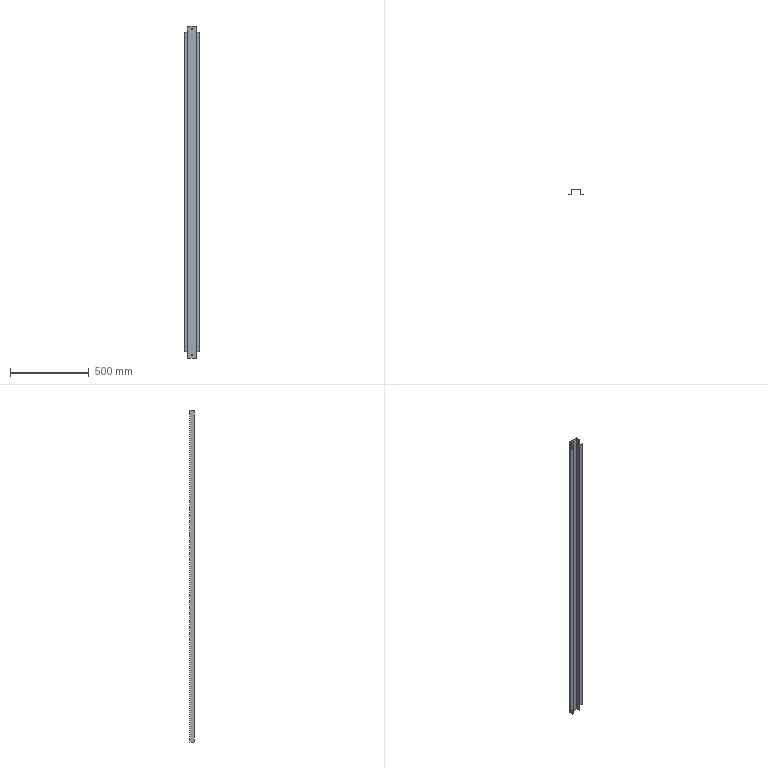Part | SolidWorks | features ICE 2, Chamfer 1, FlatPattern 1, MoveCopyBody 1, SMBaseFlange 1, SheetMetal 1 | 1 solid | 54 faces | box 100 x 30.8 x 2109 mm | volume 262992 mm3 | plane 42 | cylinder 12 | commonest cylinder face diameters 2 x4 3.6 x4 10 x4
STEP:
#1=CARTESIAN_POINT('',(0.,30.,1029.5));
#2=VERTEX_POINT('',#1);
#3=CARTESIAN_POINT('',(0.,30.,1039.5));
#4=VERTEX_POINT('',#3);
#5=CARTESIAN_POINT('',(0.,30.,1034.5));
#6=DIRECTION('',(0.,1.,0.));
#7=DIRECTION('',(-1.,0.,0.));
#8=AXIS2_PLACEMENT_3D('',#5,#6,#7);
#9=CIRCLE('',#8,5.);
#10=EDGE_CURVE('',#2,#4,#9,.T.);
#11=ORIENTED_EDGE('',*,*,#10,.F.);
#12=CARTESIAN_POINT('',(0.,30.8,1029.5));
#13=VERTEX_POINT('',#12);
#14=CARTESIAN_POINT('',(0.,20.8,1029.5));
#15=DIRECTION('',(0.,1.,0.));
#16=VECTOR('',#15,1000.);
#17=LINE('',#14,#16);
#18=EDGE_CURVE('',#2,#13,#17,.T.);
#19=ORIENTED_EDGE('',*,*,#18,.T.);
#20=CARTESIAN_POINT('',(0.,30.8,1039.5));
#21=VERTEX_POINT('',#20);
#22=CARTESIAN_POINT('',(0.,30.8,1034.5));
#23=DIRECTION('',(0.,1.,0.));
#24=DIRECTION('',(0.,0.,1.));
#25=AXIS2_PLACEMENT_3D('',#22,#23,#24);
#26=CIRCLE('',#25,5.);
#27=EDGE_CURVE('',#13,#21,#26,.T.);
#28=ORIENTED_EDGE('',*,*,#27,.T.);
#29=CARTESIAN_POINT('',(0.,20.8,1039.5));
#30=DIRECTION('',(0.,1.,0.));
#31=VECTOR('',#30,1000.);
#32=LINE('',#29,#31);
#33=EDGE_CURVE('',#4,#21,#32,.T.);
#34=ORIENTED_EDGE('',*,*,#33,.F.);
#35=EDGE_LOOP('',(#11,#19,#28,#34));
#36=FACE_OUTER_BOUND('',#35,.T.);
#37=CARTESIAN_POINT('',(0.,20.8,1034.5));
#38=DIRECTION('',(0.,1.,0.));
#39=DIRECTION('',(0.,0.,1.));
#40=AXIS2_PLACEMENT_3D('',#37,#38,#39);
#41=CYLINDRICAL_SURFACE('',#40,5.);
#42=ADVANCED_FACE('',(#36),#41,.F.);
#43=CARTESIAN_POINT('',(0.,30.,-1039.5));
#44=VERTEX_POINT('',#43);
#45=CARTESIAN_POINT('',(0.,30.,-1029.5));
#46=VERTEX_POINT('',#45);
#47=CARTESIAN_POINT('',(0.,30.,-1034.5));
#48=DIRECTION('',(0.,1.,0.));
#49=DIRECTION('',(-1.,0.,0.));
#50=AXIS2_PLACEMENT_3D('',#47,#48,#49);
#51=CIRCLE('',#50,5.);
#52=EDGE_CURVE('',#44,#46,#51,.T.);
#53=ORIENTED_EDGE('',*,*,#52,.F.);
#54=CARTESIAN_POINT('',(0.,30.8,-1039.5));
#55=VERTEX_POINT('',#54);
#56=CARTESIAN_POINT('',(0.,20.8,-1039.5));
#57=DIRECTION('',(0.,1.,0.));
#58=VECTOR('',#57,1000.);
#59=LINE('',#56,#58);
#60=EDGE_CURVE('',#44,#55,#59,.T.);
#61=ORIENTED_EDGE('',*,*,#60,.T.);
#62=CARTESIAN_POINT('',(0.,30.8,-1029.5));
#63=VERTEX_POINT('',#62);
#64=CARTESIAN_POINT('',(0.,30.8,-1034.5));
#65=DIRECTION('',(0.,1.,0.));
#66=DIRECTION('',(0.,0.,-1.));
#67=AXIS2_PLACEMENT_3D('',#64,#65,#66);
#68=CIRCLE('',#67,5.);
#69=EDGE_CURVE('',#55,#63,#68,.T.);
#70=ORIENTED_EDGE('',*,*,#69,.T.);
#71=CARTESIAN_POINT('',(0.,20.8,-1029.5));
#72=DIRECTION('',(0.,1.,0.));
#73=VECTOR('',#72,1000.);
#74=LINE('',#71,#73);
#75=EDGE_CURVE('',#46,#63,#74,.T.);
#76=ORIENTED_EDGE('',*,*,#75,.F.);
#77=EDGE_LOOP('',(#53,#61,#70,#76));
#78=FACE_OUTER_BOUND('',#77,.T.);
#79=CARTESIAN_POINT('',(0.,20.8,-1034.5));
#80=DIRECTION('',(0.,1.,0.));
#81=DIRECTION('',(0.,0.,1.));
#82=AXIS2_PLACEMENT_3D('',#79,#80,#81);
#83=CYLINDRICAL_SURFACE('',#82,5.);
#84=ADVANCED_FACE('',(#78),#83,.F.);
#85=CARTESIAN_POINT('',(-50.,0.,1014.5));
#86=VERTEX_POINT('',#85);
#87=CARTESIAN_POINT('',(-31.,0.,1014.5));
#88=VERTEX_POINT('',#87);
#89=CARTESIAN_POINT('',(-50.,0.,1014.5));
#90=DIRECTION('',(1.,0.,0.));
#91=VECTOR('',#90,1000.);
#92=LINE('',#89,#91);
#93=EDGE_CURVE('',#86,#88,#92,.T.);
#94=ORIENTED_EDGE('',*,*,#93,.T.);
#95=CARTESIAN_POINT('',(-31.,0.8,1014.5));
#96=VERTEX_POINT('',#95);
#97=CARTESIAN_POINT('',(-31.,0.,1014.5));
#98=DIRECTION('',(0.,1.,0.));
#99=VECTOR('',#98,1000.);
#100=LINE('',#97,#99);
#101=EDGE_CURVE('',#88,#96,#100,.T.);
#102=ORIENTED_EDGE('',*,*,#101,.T.);
#103=CARTESIAN_POINT('',(-50.,0.8,1014.5));
#104=VERTEX_POINT('',#103);
#105=CARTESIAN_POINT('',(-50.,0.8,1014.5));
#106=DIRECTION('',(-1.,0.,0.));
#107=VECTOR('',#106,1000.);
#108=LINE('',#105,#107);
#109=EDGE_CURVE('',#96,#104,#108,.T.);
#110=ORIENTED_EDGE('',*,*,#109,.T.);
#111=CARTESIAN_POINT('',(-50.,0.,1014.5));
#112=DIRECTION('',(0.,1.,0.));
#113=VECTOR('',#112,1000.);
#114=LINE('',#111,#113);
#115=EDGE_CURVE('',#86,#104,#114,.T.);
#116=ORIENTED_EDGE('',*,*,#115,.F.);
#117=EDGE_LOOP('',(#94,#102,#110,#116));
#118=FACE_OUTER_BOUND('',#117,.T.);
#119=CARTESIAN_POINT('',(-50.,0.,1014.5));
#120=DIRECTION('',(0.,0.,-1.));
#121=DIRECTION('',(-1.,0.,0.));
#122=AXIS2_PLACEMENT_3D('',#119,#120,#121);
#123=PLANE('',#122);
#124=ADVANCED_FACE('',(#118),#123,.F.);
#125=CARTESIAN_POINT('',(-30.,2.,1014.5));
#126=VERTEX_POINT('',#125);
#127=CARTESIAN_POINT('',(-30.,1.8,1014.5));
#128=VERTEX_POINT('',#127);
#129=CARTESIAN_POINT('',(-30.,0.8,1014.5));
#130=DIRECTION('',(0.,-1.,0.));
#131=VECTOR('',#130,1000.);
#132=LINE('',#129,#131);
#133=EDGE_CURVE('',#126,#128,#132,.T.);
#134=ORIENTED_EDGE('',*,*,#133,.T.);
#135=CARTESIAN_POINT('',(-29.2,1.8,1014.5));
#136=VERTEX_POINT('',#135);
#137=CARTESIAN_POINT('',(-30.,1.8,1014.5));
#138=DIRECTION('',(1.,0.,0.));
#139=VECTOR('',#138,1000.);
#140=LINE('',#137,#139);
#141=EDGE_CURVE('',#128,#136,#140,.T.);
#142=ORIENTED_EDGE('',*,*,#141,.T.);
#143=CARTESIAN_POINT('',(-29.2,2.,1014.5));
#144=VERTEX_POINT('',#143);
#145=CARTESIAN_POINT('',(-29.2,0.8,1014.5));
#146=DIRECTION('',(0.,-1.,0.));
#147=VECTOR('',#146,1000.);
#148=LINE('',#145,#147);
#149=EDGE_CURVE('',#144,#136,#148,.T.);
#150=ORIENTED_EDGE('',*,*,#149,.F.);
#151=CARTESIAN_POINT('',(-50.,2.,1014.5));
#152=DIRECTION('',(1.,0.,0.));
#153=VECTOR('',#152,1000.);
#154=LINE('',#151,#153);
#155=EDGE_CURVE('',#126,#144,#154,.T.);
#156=ORIENTED_EDGE('',*,*,#155,.F.);
#157=EDGE_LOOP('',(#134,#142,#150,#156));
#158=FACE_OUTER_BOUND('',#157,.T.);
#159=CARTESIAN_POINT('',(-50.,0.,1014.5));
#160=DIRECTION('',(0.,0.,-1.));
#161=DIRECTION('',(-1.,0.,0.));
#162=AXIS2_PLACEMENT_3D('',#159,#160,#161);
#163=PLANE('',#162);
#164=ADVANCED_FACE('',(#158),#163,.F.);
#165=CARTESIAN_POINT('',(-50.,0.8,-1014.5));
#166=VERTEX_POINT('',#165);
#167=CARTESIAN_POINT('',(-31.,0.8,-1014.5));
#168=VERTEX_POINT('',#167);
#169=CARTESIAN_POINT('',(-50.,0.8,-1014.5));
#170=DIRECTION('',(1.,0.,0.));
#171=VECTOR('',#170,1000.);
#172=LINE('',#169,#171);
#173=EDGE_CURVE('',#166,#168,#172,.T.);
#174=ORIENTED_EDGE('',*,*,#173,.T.);
#175=CARTESIAN_POINT('',(-31.,0.,-1014.5));
#176=VERTEX_POINT('',#175);
#177=CARTESIAN_POINT('',(-31.,0.8,-1014.5));
#178=DIRECTION('',(0.,-1.,0.));
#179=VECTOR('',#178,1000.);
#180=LINE('',#177,#179);
#181=EDGE_CURVE('',#168,#176,#180,.T.);
#182=ORIENTED_EDGE('',*,*,#181,.T.);
#183=CARTESIAN_POINT('',(-50.,0.,-1014.5));
#184=VERTEX_POINT('',#183);
#185=CARTESIAN_POINT('',(-50.,0.,-1014.5));
#186=DIRECTION('',(1.,0.,0.));
#187=VECTOR('',#186,1000.);
#188=LINE('',#185,#187);
#189=EDGE_CURVE('',#184,#176,#188,.T.);
#190=ORIENTED_EDGE('',*,*,#189,.F.);
#191=CARTESIAN_POINT('',(-50.,0.,-1014.5));
#192=DIRECTION('',(0.,-1.,0.));
#193=VECTOR('',#192,1000.);
#194=LINE('',#191,#193);
#195=EDGE_CURVE('',#166,#184,#194,.T.);
#196=ORIENTED_EDGE('',*,*,#195,.F.);
#197=EDGE_LOOP('',(#174,#182,#190,#196));
#198=FACE_OUTER_BOUND('',#197,.T.);
#199=CARTESIAN_POINT('',(-50.,0.,-1014.5));
#200=DIRECTION('',(0.,0.,1.));
#201=DIRECTION('',(1.,0.,0.));
#202=AXIS2_PLACEMENT_3D('',#199,#200,#201);
#203=PLANE('',#202);
#204=ADVANCED_FACE('',(#198),#203,.F.);
#205=CARTESIAN_POINT('',(-29.2,1.8,-1014.5));
#206=VERTEX_POINT('',#205);
#207=CARTESIAN_POINT('',(-29.2,2.,-1014.5));
#208=VERTEX_POINT('',#207);
#209=CARTESIAN_POINT('',(-29.2,0.8,-1014.5));
#210=DIRECTION('',(0.,1.,0.));
#211=VECTOR('',#210,1000.);
#212=LINE('',#209,#211);
#213=EDGE_CURVE('',#206,#208,#212,.T.);
#214=ORIENTED_EDGE('',*,*,#213,.F.);
#215=CARTESIAN_POINT('',(-30.,1.8,-1014.5));
#216=VERTEX_POINT('',#215);
#217=CARTESIAN_POINT('',(-29.2,1.8,-1014.5));
#218=DIRECTION('',(-1.,0.,0.));
#219=VECTOR('',#218,1000.);
#220=LINE('',#217,#219);
#221=EDGE_CURVE('',#206,#216,#220,.T.);
#222=ORIENTED_EDGE('',*,*,#221,.T.);
#223=CARTESIAN_POINT('',(-30.,2.,-1014.5));
#224=VERTEX_POINT('',#223);
#225=CARTESIAN_POINT('',(-30.,0.8,-1014.5));
#226=DIRECTION('',(0.,1.,0.));
#227=VECTOR('',#226,1000.);
#228=LINE('',#225,#227);
#229=EDGE_CURVE('',#216,#224,#228,.T.);
#230=ORIENTED_EDGE('',*,*,#229,.T.);
#231=CARTESIAN_POINT('',(-50.,2.,-1014.5));
#232=DIRECTION('',(1.,0.,0.));
#233=VECTOR('',#232,1000.);
#234=LINE('',#231,#233);
#235=EDGE_CURVE('',#224,#208,#234,.T.);
#236=ORIENTED_EDGE('',*,*,#235,.T.);
#237=EDGE_LOOP('',(#214,#222,#230,#236));
#238=FACE_OUTER_BOUND('',#237,.T.);
#239=CARTESIAN_POINT('',(-50.,0.,-1014.5));
#240=DIRECTION('',(0.,0.,1.));
#241=DIRECTION('',(1.,0.,0.));
#242=AXIS2_PLACEMENT_3D('',#239,#240,#241);
#243=PLANE('',#242);
#244=ADVANCED_FACE('',(#238),#243,.F.);
#245=CARTESIAN_POINT('',(29.2,1.8,1014.5));
#246=VERTEX_POINT('',#245);
#247=CARTESIAN_POINT('',(29.2,2.,1014.5));
#248=VERTEX_POINT('',#247);
#249=CARTESIAN_POINT('',(29.2,30.8,1014.5));
#250=DIRECTION('',(0.,1.,0.));
#251=VECTOR('',#250,1000.);
#252=LINE('',#249,#251);
#253=EDGE_CURVE('',#246,#248,#252,.T.);
#254=ORIENTED_EDGE('',*,*,#253,.F.);
#255=CARTESIAN_POINT('',(30.,1.8,1014.5));
#256=VERTEX_POINT('',#255);
#257=CARTESIAN_POINT('',(29.2,1.8,1014.5));
#258=DIRECTION('',(1.,0.,0.));
#259=VECTOR('',#258,1000.);
#260=LINE('',#257,#259);
#261=EDGE_CURVE('',#246,#256,#260,.T.);
#262=ORIENTED_EDGE('',*,*,#261,.T.);
#263=CARTESIAN_POINT('',(30.,2.,1014.5));
#264=VERTEX_POINT('',#263);
#265=CARTESIAN_POINT('',(30.,30.8,1014.5));
#266=DIRECTION('',(0.,1.,0.));
#267=VECTOR('',#266,1000.);
#268=LINE('',#265,#267);
#269=EDGE_CURVE('',#256,#264,#268,.T.);
#270=ORIENTED_EDGE('',*,*,#269,.T.);
#271=CARTESIAN_POINT('',(-50.,2.,1014.5));
#272=DIRECTION('',(1.,0.,0.));
#273=VECTOR('',#272,1000.);
#274=LINE('',#271,#273);
#275=EDGE_CURVE('',#248,#264,#274,.T.);
#276=ORIENTED_EDGE('',*,*,#275,.F.);
#277=EDGE_LOOP('',(#254,#262,#270,#276));
#278=FACE_OUTER_BOUND('',#277,.T.);
#279=CARTESIAN_POINT('',(-50.,0.,1014.5));
#280=DIRECTION('',(0.,0.,-1.));
#281=DIRECTION('',(-1.,0.,0.));
#282=AXIS2_PLACEMENT_3D('',#279,#280,#281);
#283=PLANE('',#282);
#284=ADVANCED_FACE('',(#278),#283,.F.);
#285=CARTESIAN_POINT('',(50.,0.8,1014.5));
#286=VERTEX_POINT('',#285);
#287=CARTESIAN_POINT('',(31.,0.8,1014.5));
#288=VERTEX_POINT('',#287);
#289=CARTESIAN_POINT('',(30.,0.8,1014.5));
#290=DIRECTION('',(-1.,0.,0.));
#291=VECTOR('',#290,1000.);
#292=LINE('',#289,#291);
#293=EDGE_CURVE('',#286,#288,#292,.T.);
#294=ORIENTED_EDGE('',*,*,#293,.T.);
#295=CARTESIAN_POINT('',(31.,0.,1014.5));
#296=VERTEX_POINT('',#295);
#297=CARTESIAN_POINT('',(31.,0.8,1014.5));
#298=DIRECTION('',(0.,-1.,0.));
#299=VECTOR('',#298,1000.);
#300=LINE('',#297,#299);
#301=EDGE_CURVE('',#288,#296,#300,.T.);
#302=ORIENTED_EDGE('',*,*,#301,.T.);
#303=CARTESIAN_POINT('',(50.,0.,1014.5));
#304=VERTEX_POINT('',#303);
#305=CARTESIAN_POINT('',(-50.,0.,1014.5));
#306=DIRECTION('',(1.,0.,0.));
#307=VECTOR('',#306,1000.);
#308=LINE('',#305,#307);
#309=EDGE_CURVE('',#296,#304,#308,.T.);
#310=ORIENTED_EDGE('',*,*,#309,.T.);
#311=CARTESIAN_POINT('',(50.,0.,1014.5));
#312=DIRECTION('',(0.,1.,0.));
#313=VECTOR('',#312,1000.);
#314=LINE('',#311,#313);
#315=EDGE_CURVE('',#304,#286,#314,.T.);
#316=ORIENTED_EDGE('',*,*,#315,.T.);
#317=EDGE_LOOP('',(#294,#302,#310,#316));
#318=FACE_OUTER_BOUND('',#317,.T.);
#319=CARTESIAN_POINT('',(-50.,0.,1014.5));
#320=DIRECTION('',(0.,0.,-1.));
#321=DIRECTION('',(-1.,0.,0.));
#322=AXIS2_PLACEMENT_3D('',#319,#320,#321);
#323=PLANE('',#322);
#324=ADVANCED_FACE('',(#318),#323,.F.);
#325=CARTESIAN_POINT('',(30.,2.,-1014.5));
#326=VERTEX_POINT('',#325);
#327=CARTESIAN_POINT('',(30.,1.8,-1014.5));
#328=VERTEX_POINT('',#327);
#329=CARTESIAN_POINT('',(30.,30.8,-1014.5));
#330=DIRECTION('',(0.,-1.,0.));
#331=VECTOR('',#330,1000.);
#332=LINE('',#329,#331);
#333=EDGE_CURVE('',#326,#328,#332,.T.);
#334=ORIENTED_EDGE('',*,*,#333,.T.);
#335=CARTESIAN_POINT('',(29.2,1.8,-1014.5));
#336=VERTEX_POINT('',#335);
#337=CARTESIAN_POINT('',(30.,1.8,-1014.5));
#338=DIRECTION('',(-1.,0.,0.));
#339=VECTOR('',#338,1000.);
#340=LINE('',#337,#339);
#341=EDGE_CURVE('',#328,#336,#340,.T.);
#342=ORIENTED_EDGE('',*,*,#341,.T.);
#343=CARTESIAN_POINT('',(29.2,2.,-1014.5));
#344=VERTEX_POINT('',#343);
#345=CARTESIAN_POINT('',(29.2,30.8,-1014.5));
#346=DIRECTION('',(0.,-1.,0.));
#347=VECTOR('',#346,1000.);
#348=LINE('',#345,#347);
#349=EDGE_CURVE('',#344,#336,#348,.T.);
#350=ORIENTED_EDGE('',*,*,#349,.F.);
#351=CARTESIAN_POINT('',(-50.,2.,-1014.5));
#352=DIRECTION('',(1.,0.,0.));
#353=VECTOR('',#352,1000.);
#354=LINE('',#351,#353);
#355=EDGE_CURVE('',#344,#326,#354,.T.);
#356=ORIENTED_EDGE('',*,*,#355,.T.);
#357=EDGE_LOOP('',(#334,#342,#350,#356));
#358=FACE_OUTER_BOUND('',#357,.T.);
#359=CARTESIAN_POINT('',(-50.,0.,-1014.5));
#360=DIRECTION('',(0.,0.,1.));
#361=DIRECTION('',(1.,0.,0.));
#362=AXIS2_PLACEMENT_3D('',#359,#360,#361);
#363=PLANE('',#362);
#364=ADVANCED_FACE('',(#358),#363,.F.);
#365=CARTESIAN_POINT('',(31.,0.,-1014.5));
#366=VERTEX_POINT('',#365);
#367=CARTESIAN_POINT('',(50.,0.,-1014.5));
#368=VERTEX_POINT('',#367);
#369=CARTESIAN_POINT('',(-50.,0.,-1014.5));
#370=DIRECTION('',(1.,0.,0.));
#371=VECTOR('',#370,1000.);
#372=LINE('',#369,#371);
#373=EDGE_CURVE('',#366,#368,#372,.T.);
#374=ORIENTED_EDGE('',*,*,#373,.F.);
#375=CARTESIAN_POINT('',(31.,0.8,-1014.5));
#376=VERTEX_POINT('',#375);
#377=CARTESIAN_POINT('',(31.,0.,-1014.5));
#378=DIRECTION('',(0.,1.,0.));
#379=VECTOR('',#378,1000.);
#380=LINE('',#377,#379);
#381=EDGE_CURVE('',#366,#376,#380,.T.);
#382=ORIENTED_EDGE('',*,*,#381,.T.);
#383=CARTESIAN_POINT('',(50.,0.8,-1014.5));
#384=VERTEX_POINT('',#383);
#385=CARTESIAN_POINT('',(30.,0.8,-1014.5));
#386=DIRECTION('',(1.,0.,0.));
#387=VECTOR('',#386,1000.);
#388=LINE('',#385,#387);
#389=EDGE_CURVE('',#376,#384,#388,.T.);
#390=ORIENTED_EDGE('',*,*,#389,.T.);
#391=CARTESIAN_POINT('',(50.,0.,-1014.5));
#392=DIRECTION('',(0.,-1.,0.));
#393=VECTOR('',#392,1000.);
#394=LINE('',#391,#393);
#395=EDGE_CURVE('',#384,#368,#394,.T.);
#396=ORIENTED_EDGE('',*,*,#395,.T.);
#397=EDGE_LOOP('',(#374,#382,#390,#396));
#398=FACE_OUTER_BOUND('',#397,.T.);
#399=CARTESIAN_POINT('',(-50.,0.,-1014.5));
#400=DIRECTION('',(0.,0.,1.));
#401=DIRECTION('',(1.,0.,0.));
#402=AXIS2_PLACEMENT_3D('',#399,#400,#401);
#403=PLANE('',#402);
#404=ADVANCED_FACE('',(#398),#403,.F.);
#405=CARTESIAN_POINT('',(-30.,7.,1054.5));
#406=VERTEX_POINT('',#405);
#407=CARTESIAN_POINT('',(-30.,29.,1054.5));
#408=VERTEX_POINT('',#407);
#409=CARTESIAN_POINT('',(-30.,0.8,1054.5));
#410=DIRECTION('',(0.,1.,0.));
#411=VECTOR('',#410,1000.);
#412=LINE('',#409,#411);
#413=EDGE_CURVE('',#406,#408,#412,.T.);
#414=ORIENTED_EDGE('',*,*,#413,.F.);
#415=CARTESIAN_POINT('',(-29.2,7.,1054.5));
#416=VERTEX_POINT('',#415);
#417=CARTESIAN_POINT('',(-29.2,7.,1054.5));
#418=DIRECTION('',(1.,0.,0.));
#419=VECTOR('',#418,1000.);
#420=LINE('',#417,#419);
#421=EDGE_CURVE('',#406,#416,#420,.T.);
#422=ORIENTED_EDGE('',*,*,#421,.T.);
#423=CARTESIAN_POINT('',(-29.2,29.,1054.5));
#424=VERTEX_POINT('',#423);
#425=CARTESIAN_POINT('',(-29.2,0.8,1054.5));
#426=DIRECTION('',(0.,1.,0.));
#427=VECTOR('',#426,1000.);
#428=LINE('',#425,#427);
#429=EDGE_CURVE('',#416,#424,#428,.T.);
#430=ORIENTED_EDGE('',*,*,#429,.T.);
#431=CARTESIAN_POINT('',(-29.2,29.,1054.5));
#432=DIRECTION('',(-1.,0.,0.));
#433=VECTOR('',#432,1000.);
#434=LINE('',#431,#433);
#435=EDGE_CURVE('',#424,#408,#434,.T.);
#436=ORIENTED_EDGE('',*,*,#435,.T.);
#437=EDGE_LOOP('',(#414,#422,#430,#436));
#438=FACE_OUTER_BOUND('',#437,.T.);
#439=CARTESIAN_POINT('',(-31.,0.,1054.5));
#440=DIRECTION('',(0.,0.,1.));
#441=DIRECTION('',(1.,0.,0.));
#442=AXIS2_PLACEMENT_3D('',#439,#440,#441);
#443=PLANE('',#442);
#444=ADVANCED_FACE('',(#438),#443,.T.);
#445=CARTESIAN_POINT('',(-28.2,30.8,1054.5));
#446=VERTEX_POINT('',#445);
#447=CARTESIAN_POINT('',(-28.2,30.,1054.5));
#448=VERTEX_POINT('',#447);
#449=CARTESIAN_POINT('',(-28.2,30.8,1054.5));
#450=DIRECTION('',(0.,-1.,0.));
#451=VECTOR('',#450,1000.);
#452=LINE('',#449,#451);
#453=EDGE_CURVE('',#446,#448,#452,.T.);
#454=ORIENTED_EDGE('',*,*,#453,.F.);
#455=CARTESIAN_POINT('',(-28.2,29.,1054.5));
#456=DIRECTION('',(0.,0.,-1.));
#457=DIRECTION('',(1.,0.,0.));
#458=AXIS2_PLACEMENT_3D('',#455,#456,#457);
#459=CIRCLE('',#458,1.8);
#460=EDGE_CURVE('',#408,#446,#459,.T.);
#461=ORIENTED_EDGE('',*,*,#460,.F.);
#462=ORIENTED_EDGE('',*,*,#435,.F.);
#463=CARTESIAN_POINT('',(-28.2,29.,1054.5));
#464=DIRECTION('',(0.,0.,-1.));
#465=DIRECTION('',(1.,0.,0.));
#466=AXIS2_PLACEMENT_3D('',#463,#464,#465);
#467=CIRCLE('',#466,1.);
#468=EDGE_CURVE('',#424,#448,#467,.T.);
#469=ORIENTED_EDGE('',*,*,#468,.T.);
#470=EDGE_LOOP('',(#454,#461,#462,#469));
#471=FACE_OUTER_BOUND('',#470,.T.);
#472=CARTESIAN_POINT('',(-28.2,30.8,1054.5));
#473=DIRECTION('',(0.,0.,1.));
#474=DIRECTION('',(1.,0.,0.));
#475=AXIS2_PLACEMENT_3D('',#472,#473,#474);
#476=PLANE('',#475);
#477=ADVANCED_FACE('',(#471),#476,.T.);
#478=CARTESIAN_POINT('',(28.2,30.8,1054.5));
#479=VERTEX_POINT('',#478);
#480=CARTESIAN_POINT('',(-30.,30.8,1054.5));
#481=DIRECTION('',(1.,0.,0.));
#482=VECTOR('',#481,1000.);
#483=LINE('',#480,#482);
#484=EDGE_CURVE('',#446,#479,#483,.T.);
#485=ORIENTED_EDGE('',*,*,#484,.F.);
#486=ORIENTED_EDGE('',*,*,#453,.T.);
#487=CARTESIAN_POINT('',(28.2,30.,1054.5));
#488=VERTEX_POINT('',#487);
#489=CARTESIAN_POINT('',(-30.,30.,1054.5));
#490=DIRECTION('',(1.,0.,0.));
#491=VECTOR('',#490,1000.);
#492=LINE('',#489,#491);
#493=EDGE_CURVE('',#448,#488,#492,.T.);
#494=ORIENTED_EDGE('',*,*,#493,.T.);
#495=CARTESIAN_POINT('',(28.2,30.,1054.5));
#496=DIRECTION('',(0.,1.,0.));
#497=VECTOR('',#496,1000.);
#498=LINE('',#495,#497);
#499=EDGE_CURVE('',#488,#479,#498,.T.);
#500=ORIENTED_EDGE('',*,*,#499,.T.);
#501=EDGE_LOOP('',(#485,#486,#494,#500));
#502=FACE_OUTER_BOUND('',#501,.T.);
#503=CARTESIAN_POINT('',(-29.2,29.,1054.5));
#504=DIRECTION('',(0.,0.,1.));
#505=DIRECTION('',(1.,0.,0.));
#506=AXIS2_PLACEMENT_3D('',#503,#504,#505);
#507=PLANE('',#506);
#508=ADVANCED_FACE('',(#502),#507,.T.);
#509=CARTESIAN_POINT('',(-30.,29.,-1054.5));
#510=VERTEX_POINT('',#509);
#511=CARTESIAN_POINT('',(-29.2,29.,-1054.5));
#512=VERTEX_POINT('',#511);
#513=CARTESIAN_POINT('',(-30.,29.,-1054.5));
#514=DIRECTION('',(1.,0.,0.));
#515=VECTOR('',#514,1000.);
#516=LINE('',#513,#515);
#517=EDGE_CURVE('',#510,#512,#516,.T.);
#518=ORIENTED_EDGE('',*,*,#517,.F.);
#519=CARTESIAN_POINT('',(-28.2,30.8,-1054.5));
#520=VERTEX_POINT('',#519);
#521=CARTESIAN_POINT('',(-28.2,29.,-1054.5));
#522=DIRECTION('',(0.,0.,-1.));
#523=DIRECTION('',(1.,0.,0.));
#524=AXIS2_PLACEMENT_3D('',#521,#522,#523);
#525=CIRCLE('',#524,1.8);
#526=EDGE_CURVE('',#510,#520,#525,.T.);
#527=ORIENTED_EDGE('',*,*,#526,.T.);
#528=CARTESIAN_POINT('',(-28.2,30.,-1054.5));
#529=VERTEX_POINT('',#528);
#530=CARTESIAN_POINT('',(-28.2,30.,-1054.5));
#531=DIRECTION('',(0.,1.,0.));
#532=VECTOR('',#531,1000.);
#533=LINE('',#530,#532);
#534=EDGE_CURVE('',#529,#520,#533,.T.);
#535=ORIENTED_EDGE('',*,*,#534,.F.);
#536=CARTESIAN_POINT('',(-28.2,29.,-1054.5));
#537=DIRECTION('',(0.,0.,-1.));
#538=DIRECTION('',(1.,0.,0.));
#539=AXIS2_PLACEMENT_3D('',#536,#537,#538);
#540=CIRCLE('',#539,1.);
#541=EDGE_CURVE('',#512,#529,#540,.T.);
#542=ORIENTED_EDGE('',*,*,#541,.F.);
#543=EDGE_LOOP('',(#518,#527,#535,#542));
#544=FACE_OUTER_BOUND('',#543,.T.);
#545=CARTESIAN_POINT('',(-30.,29.,-1054.5));
#546=DIRECTION('',(0.,0.,-1.));
#547=DIRECTION('',(-1.,0.,0.));
#548=AXIS2_PLACEMENT_3D('',#545,#546,#547);
#549=PLANE('',#548);
#550=ADVANCED_FACE('',(#544),#549,.T.);
#551=CARTESIAN_POINT('',(-29.2,7.,-1054.5));
#552=VERTEX_POINT('',#551);
#553=CARTESIAN_POINT('',(-29.2,0.8,-1054.5));
#554=DIRECTION('',(0.,1.,0.));
#555=VECTOR('',#554,1000.);
#556=LINE('',#553,#555);
#557=EDGE_CURVE('',#552,#512,#556,.T.);
#558=ORIENTED_EDGE('',*,*,#557,.F.);
#559=CARTESIAN_POINT('',(-30.,7.,-1054.5));
#560=VERTEX_POINT('',#559);
#561=CARTESIAN_POINT('',(-30.,7.,-1054.5));
#562=DIRECTION('',(-1.,0.,0.));
#563=VECTOR('',#562,1000.);
#564=LINE('',#561,#563);
#565=EDGE_CURVE('',#552,#560,#564,.T.);
#566=ORIENTED_EDGE('',*,*,#565,.T.);
#567=CARTESIAN_POINT('',(-30.,0.8,-1054.5));
#568=DIRECTION('',(0.,1.,0.));
#569=VECTOR('',#568,1000.);
#570=LINE('',#567,#569);
#571=EDGE_CURVE('',#560,#510,#570,.T.);
#572=ORIENTED_EDGE('',*,*,#571,.T.);
#573=ORIENTED_EDGE('',*,*,#517,.T.);
#574=EDGE_LOOP('',(#558,#566,#572,#573));
#575=FACE_OUTER_BOUND('',#574,.T.);
#576=CARTESIAN_POINT('',(-28.2,30.,-1054.5));
#577=DIRECTION('',(0.,0.,-1.));
#578=DIRECTION('',(-1.,0.,0.));
#579=AXIS2_PLACEMENT_3D('',#576,#577,#578);
#580=PLANE('',#579);
#581=ADVANCED_FACE('',(#575),#580,.T.);
#582=CARTESIAN_POINT('',(30.,29.,1054.5));
#583=VERTEX_POINT('',#582);
#584=CARTESIAN_POINT('',(29.2,29.,1054.5));
#585=VERTEX_POINT('',#584);
#586=CARTESIAN_POINT('',(30.,29.,1054.5));
#587=DIRECTION('',(-1.,0.,0.));
#588=VECTOR('',#587,1000.);
#589=LINE('',#586,#588);
#590=EDGE_CURVE('',#583,#585,#589,.T.);
#591=ORIENTED_EDGE('',*,*,#590,.F.);
#592=CARTESIAN_POINT('',(28.2,29.,1054.5));
#593=DIRECTION('',(0.,0.,-1.));
#594=DIRECTION('',(1.,0.,0.));
#595=AXIS2_PLACEMENT_3D('',#592,#593,#594);
#596=CIRCLE('',#595,1.8);
#597=EDGE_CURVE('',#479,#583,#596,.T.);
#598=ORIENTED_EDGE('',*,*,#597,.F.);
#599=ORIENTED_EDGE('',*,*,#499,.F.);
#600=CARTESIAN_POINT('',(28.2,29.,1054.5));
#601=DIRECTION('',(0.,0.,-1.));
#602=DIRECTION('',(1.,0.,0.));
#603=AXIS2_PLACEMENT_3D('',#600,#601,#602);
#604=CIRCLE('',#603,1.);
#605=EDGE_CURVE('',#488,#585,#604,.T.);
#606=ORIENTED_EDGE('',*,*,#605,.T.);
#607=EDGE_LOOP('',(#591,#598,#599,#606));
#608=FACE_OUTER_BOUND('',#607,.T.);
#609=CARTESIAN_POINT('',(30.,29.,1054.5));
#610=DIRECTION('',(0.,0.,1.));
#611=DIRECTION('',(1.,0.,0.));
#612=AXIS2_PLACEMENT_3D('',#609,#610,#611);
#613=PLANE('',#612);
#614=ADVANCED_FACE('',(#608),#613,.T.);
#615=CARTESIAN_POINT('',(29.2,7.,1054.5));
#616=VERTEX_POINT('',#615);
#617=CARTESIAN_POINT('',(29.2,30.8,1054.5));
#618=DIRECTION('',(0.,-1.,0.));
#619=VECTOR('',#618,1000.);
#620=LINE('',#617,#619);
#621=EDGE_CURVE('',#585,#616,#620,.T.);
#622=ORIENTED_EDGE('',*,*,#621,.T.);
#623=CARTESIAN_POINT('',(30.,7.,1054.5));
#624=VERTEX_POINT('',#623);
#625=CARTESIAN_POINT('',(30.,7.,1054.5));
#626=DIRECTION('',(1.,0.,0.));
#627=VECTOR('',#626,1000.);
#628=LINE('',#625,#627);
#629=EDGE_CURVE('',#616,#624,#628,.T.);
#630=ORIENTED_EDGE('',*,*,#629,.T.);
#631=CARTESIAN_POINT('',(30.,30.8,1054.5));
#632=DIRECTION('',(0.,-1.,0.));
#633=VECTOR('',#632,1000.);
#634=LINE('',#631,#633);
#635=EDGE_CURVE('',#583,#624,#634,.T.);
#636=ORIENTED_EDGE('',*,*,#635,.F.);
#637=ORIENTED_EDGE('',*,*,#590,.T.);
#638=EDGE_LOOP('',(#622,#630,#636,#637));
#639=FACE_OUTER_BOUND('',#638,.T.);
#640=CARTESIAN_POINT('',(28.2,30.,1054.5));
#641=DIRECTION('',(0.,0.,1.));
#642=DIRECTION('',(1.,0.,0.));
#643=AXIS2_PLACEMENT_3D('',#640,#641,#642);
#644=PLANE('',#643);
#645=ADVANCED_FACE('',(#639),#644,.T.);
#646=CARTESIAN_POINT('',(28.2,30.8,-1054.5));
#647=VERTEX_POINT('',#646);
#648=CARTESIAN_POINT('',(28.2,30.,-1054.5));
#649=VERTEX_POINT('',#648);
#650=CARTESIAN_POINT('',(28.2,30.8,-1054.5));
#651=DIRECTION('',(0.,-1.,0.));
#652=VECTOR('',#651,1000.);
#653=LINE('',#650,#652);
#654=EDGE_CURVE('',#647,#649,#653,.T.);
#655=ORIENTED_EDGE('',*,*,#654,.F.);
#656=CARTESIAN_POINT('',(30.,29.,-1054.5));
#657=VERTEX_POINT('',#656);
#658=CARTESIAN_POINT('',(28.2,29.,-1054.5));
#659=DIRECTION('',(0.,0.,-1.));
#660=DIRECTION('',(1.,0.,0.));
#661=AXIS2_PLACEMENT_3D('',#658,#659,#660);
#662=CIRCLE('',#661,1.8);
#663=EDGE_CURVE('',#647,#657,#662,.T.);
#664=ORIENTED_EDGE('',*,*,#663,.T.);
#665=CARTESIAN_POINT('',(29.2,29.,-1054.5));
#666=VERTEX_POINT('',#665);
#667=CARTESIAN_POINT('',(29.2,29.,-1054.5));
#668=DIRECTION('',(1.,0.,0.));
#669=VECTOR('',#668,1000.);
#670=LINE('',#667,#669);
#671=EDGE_CURVE('',#666,#657,#670,.T.);
#672=ORIENTED_EDGE('',*,*,#671,.F.);
#673=CARTESIAN_POINT('',(28.2,29.,-1054.5));
#674=DIRECTION('',(0.,0.,-1.));
#675=DIRECTION('',(1.,0.,0.));
#676=AXIS2_PLACEMENT_3D('',#673,#674,#675);
#677=CIRCLE('',#676,1.);
#678=EDGE_CURVE('',#649,#666,#677,.T.);
#679=ORIENTED_EDGE('',*,*,#678,.F.);
#680=EDGE_LOOP('',(#655,#664,#672,#679));
#681=FACE_OUTER_BOUND('',#680,.T.);
#682=CARTESIAN_POINT('',(28.2,30.8,-1054.5));
#683=DIRECTION('',(0.,0.,-1.));
#684=DIRECTION('',(-1.,0.,0.));
#685=AXIS2_PLACEMENT_3D('',#682,#683,#684);
#686=PLANE('',#685);
#687=ADVANCED_FACE('',(#681),#686,.T.);
#688=CARTESIAN_POINT('',(-30.,30.8,-1054.5));
#689=DIRECTION('',(1.,0.,0.));
#690=VECTOR('',#689,1000.);
#691=LINE('',#688,#690);
#692=EDGE_CURVE('',#520,#647,#691,.T.);
#693=ORIENTED_EDGE('',*,*,#692,.T.);
#694=ORIENTED_EDGE('',*,*,#654,.T.);
#695=CARTESIAN_POINT('',(-30.,30.,-1054.5));
#696=DIRECTION('',(1.,0.,0.));
#697=VECTOR('',#696,1000.);
#698=LINE('',#695,#697);
#699=EDGE_CURVE('',#529,#649,#698,.T.);
#700=ORIENTED_EDGE('',*,*,#699,.F.);
#701=ORIENTED_EDGE('',*,*,#534,.T.);
#702=EDGE_LOOP('',(#693,#694,#700,#701));
#703=FACE_OUTER_BOUND('',#702,.T.);
#704=CARTESIAN_POINT('',(29.2,29.,-1054.5));
#705=DIRECTION('',(0.,0.,-1.));
#706=DIRECTION('',(-1.,0.,0.));
#707=AXIS2_PLACEMENT_3D('',#704,#705,#706);
#708=PLANE('',#707);
#709=ADVANCED_FACE('',(#703),#708,.T.);
#710=CARTESIAN_POINT('',(30.,7.,-1054.5));
#711=VERTEX_POINT('',#710);
#712=CARTESIAN_POINT('',(30.,30.8,-1054.5));
#713=DIRECTION('',(0.,-1.,0.));
#714=VECTOR('',#713,1000.);
#715=LINE('',#712,#714);
#716=EDGE_CURVE('',#657,#711,#715,.T.);
#717=ORIENTED_EDGE('',*,*,#716,.T.);
#718=CARTESIAN_POINT('',(29.2,7.,-1054.5));
#719=VERTEX_POINT('',#718);
#720=CARTESIAN_POINT('',(29.2,7.,-1054.5));
#721=DIRECTION('',(-1.,0.,0.));
#722=VECTOR('',#721,1000.);
#723=LINE('',#720,#722);
#724=EDGE_CURVE('',#711,#719,#723,.T.);
#725=ORIENTED_EDGE('',*,*,#724,.T.);
#726=CARTESIAN_POINT('',(29.2,30.8,-1054.5));
#727=DIRECTION('',(0.,-1.,0.));
#728=VECTOR('',#727,1000.);
#729=LINE('',#726,#728);
#730=EDGE_CURVE('',#666,#719,#729,.T.);
#731=ORIENTED_EDGE('',*,*,#730,.F.);
#732=ORIENTED_EDGE('',*,*,#671,.T.);
#733=EDGE_LOOP('',(#717,#725,#731,#732));
#734=FACE_OUTER_BOUND('',#733,.T.);
#735=CARTESIAN_POINT('',(31.,0.,-1054.5));
#736=DIRECTION('',(0.,0.,-1.));
#737=DIRECTION('',(-1.,0.,0.));
#738=AXIS2_PLACEMENT_3D('',#735,#736,#737);
#739=PLANE('',#738);
#740=ADVANCED_FACE('',(#734),#739,.T.);
#741=CARTESIAN_POINT('',(50.,0.,1054.5));
#742=DIRECTION('',(0.,0.,-1.));
#743=VECTOR('',#742,1000.);
#744=LINE('',#741,#743);
#745=EDGE_CURVE('',#304,#368,#744,.T.);
#746=ORIENTED_EDGE('',*,*,#745,.F.);
#747=ORIENTED_EDGE('',*,*,#309,.F.);
#748=CARTESIAN_POINT('',(31.,0.,1054.5));
#749=DIRECTION('',(0.,0.,-1.));
#750=VECTOR('',#749,1000.);
#751=LINE('',#748,#750);
#752=EDGE_CURVE('',#296,#366,#751,.T.);
#753=ORIENTED_EDGE('',*,*,#752,.T.);
#754=ORIENTED_EDGE('',*,*,#373,.T.);
#755=EDGE_LOOP('',(#746,#747,#753,#754));
#756=FACE_OUTER_BOUND('',#755,.T.);
#757=CARTESIAN_POINT('',(30.,0.,1054.5));
#758=DIRECTION('',(0.,1.,0.));
#759=DIRECTION('',(-1.,0.,0.));
#760=AXIS2_PLACEMENT_3D('',#757,#758,#759);
#761=PLANE('',#760);
#762=ADVANCED_FACE('',(#756),#761,.F.);
#763=ORIENTED_EDGE('',*,*,#315,.F.);
#764=ORIENTED_EDGE('',*,*,#745,.T.);
#765=ORIENTED_EDGE('',*,*,#395,.F.);
#766=CARTESIAN_POINT('',(50.,0.8,1054.5));
#767=DIRECTION('',(0.,0.,-1.));
#768=VECTOR('',#767,1000.);
#769=LINE('',#766,#768);
#770=EDGE_CURVE('',#286,#384,#769,.T.);
#771=ORIENTED_EDGE('',*,*,#770,.F.);
#772=EDGE_LOOP('',(#763,#764,#765,#771));
#773=FACE_OUTER_BOUND('',#772,.T.);
#774=CARTESIAN_POINT('',(50.,0.8,1054.5));
#775=DIRECTION('',(1.,0.,0.));
#776=DIRECTION('',(0.,0.,-1.));
#777=AXIS2_PLACEMENT_3D('',#774,#775,#776);
#778=PLANE('',#777);
#779=ADVANCED_FACE('',(#773),#778,.T.);
#780=ORIENTED_EDGE('',*,*,#293,.F.);
#781=ORIENTED_EDGE('',*,*,#770,.T.);
#782=ORIENTED_EDGE('',*,*,#389,.F.);
#783=CARTESIAN_POINT('',(31.,0.8,1054.5));
#784=DIRECTION('',(0.,0.,-1.));
#785=VECTOR('',#784,1000.);
#786=LINE('',#783,#785);
#787=EDGE_CURVE('',#288,#376,#786,.T.);
#788=ORIENTED_EDGE('',*,*,#787,.F.);
#789=EDGE_LOOP('',(#780,#781,#782,#788));
#790=FACE_OUTER_BOUND('',#789,.T.);
#791=CARTESIAN_POINT('',(30.,0.8,1054.5));
#792=DIRECTION('',(0.,1.,0.));
#793=DIRECTION('',(-1.,0.,0.));
#794=AXIS2_PLACEMENT_3D('',#791,#792,#793);
#795=PLANE('',#794);
#796=ADVANCED_FACE('',(#790),#795,.T.);
#797=CARTESIAN_POINT('',(31.,1.8,1014.5));
#798=DIRECTION('',(0.,0.,-1.));
#799=DIRECTION('',(-1.,0.,0.));
#800=AXIS2_PLACEMENT_3D('',#797,#798,#799);
#801=CIRCLE('',#800,1.);
#802=EDGE_CURVE('',#288,#256,#801,.T.);
#803=ORIENTED_EDGE('',*,*,#802,.F.);
#804=ORIENTED_EDGE('',*,*,#787,.T.);
#805=CARTESIAN_POINT('',(31.,1.8,-1014.5));
#806=DIRECTION('',(0.,0.,1.));
#807=DIRECTION('',(1.,0.,0.));
#808=AXIS2_PLACEMENT_3D('',#805,#806,#807);
#809=CIRCLE('',#808,1.);
#810=EDGE_CURVE('',#328,#376,#809,.T.);
#811=ORIENTED_EDGE('',*,*,#810,.F.);
#812=CARTESIAN_POINT('',(30.,1.8,1054.5));
#813=DIRECTION('',(0.,0.,-1.));
#814=VECTOR('',#813,1000.);
#815=LINE('',#812,#814);
#816=EDGE_CURVE('',#256,#328,#815,.T.);
#817=ORIENTED_EDGE('',*,*,#816,.F.);
#818=EDGE_LOOP('',(#803,#804,#811,#817));
#819=FACE_OUTER_BOUND('',#818,.T.);
#820=CARTESIAN_POINT('',(31.,1.8,1054.5));
#821=DIRECTION('',(0.,0.,-1.));
#822=DIRECTION('',(-1.,0.,0.));
#823=AXIS2_PLACEMENT_3D('',#820,#821,#822);
#824=CYLINDRICAL_SURFACE('',#823,1.);
#825=ADVANCED_FACE('',(#819),#824,.F.);
#826=CARTESIAN_POINT('',(30.,2.,-1049.5));
#827=VERTEX_POINT('',#826);
#828=CARTESIAN_POINT('',(30.,2.,1054.5));
#829=DIRECTION('',(0.,0.,1.));
#830=VECTOR('',#829,1000.);
#831=LINE('',#828,#830);
#832=EDGE_CURVE('',#827,#326,#831,.T.);
#833=ORIENTED_EDGE('',*,*,#832,.F.);
#834=CARTESIAN_POINT('',(30.,-1035.6,-11.9));
#835=DIRECTION('',(0.,0.7071,-0.7071));
#836=VECTOR('',#835,1000.);
#837=LINE('',#834,#836);
#838=EDGE_CURVE('',#827,#711,#837,.T.);
#839=ORIENTED_EDGE('',*,*,#838,.T.);
#840=ORIENTED_EDGE('',*,*,#716,.F.);
#841=CARTESIAN_POINT('',(30.,29.,1054.5));
#842=DIRECTION('',(0.,0.,-1.));
#843=VECTOR('',#842,1000.);
#844=LINE('',#841,#843);
#845=EDGE_CURVE('',#583,#657,#844,.T.);
#846=ORIENTED_EDGE('',*,*,#845,.F.);
#847=ORIENTED_EDGE('',*,*,#635,.T.);
#848=CARTESIAN_POINT('',(30.,2.,1049.5));
#849=VERTEX_POINT('',#848);
#850=CARTESIAN_POINT('',(30.,18.9,1066.4));
#851=DIRECTION('',(0.,-0.7071,-0.7071));
#852=VECTOR('',#851,1000.);
#853=LINE('',#850,#852);
#854=EDGE_CURVE('',#624,#849,#853,.T.);
#855=ORIENTED_EDGE('',*,*,#854,.T.);
#856=CARTESIAN_POINT('',(30.,2.,1054.5));
#857=DIRECTION('',(0.,0.,1.));
#858=VECTOR('',#857,1000.);
#859=LINE('',#856,#858);
#860=EDGE_CURVE('',#264,#849,#859,.T.);
#861=ORIENTED_EDGE('',*,*,#860,.F.);
#862=ORIENTED_EDGE('',*,*,#269,.F.);
#863=ORIENTED_EDGE('',*,*,#816,.T.);
#864=ORIENTED_EDGE('',*,*,#333,.F.);
#865=EDGE_LOOP('',(#833,#839,#840,#846,#847,#855,#861,#862,#863,#864));
#866=FACE_OUTER_BOUND('',#865,.T.);
#867=CARTESIAN_POINT('',(30.,30.8,1054.5));
#868=DIRECTION('',(1.,0.,0.));
#869=DIRECTION('',(0.,1.,0.));
#870=AXIS2_PLACEMENT_3D('',#867,#868,#869);
#871=PLANE('',#870);
#872=ADVANCED_FACE('',(#866),#871,.T.);
#873=ORIENTED_EDGE('',*,*,#663,.F.);
#874=CARTESIAN_POINT('',(28.2,30.8,1054.5));
#875=DIRECTION('',(0.,0.,-1.));
#876=VECTOR('',#875,1000.);
#877=LINE('',#874,#876);
#878=EDGE_CURVE('',#479,#647,#877,.T.);
#879=ORIENTED_EDGE('',*,*,#878,.F.);
#880=ORIENTED_EDGE('',*,*,#597,.T.);
#881=ORIENTED_EDGE('',*,*,#845,.T.);
#882=EDGE_LOOP('',(#873,#879,#880,#881));
#883=FACE_OUTER_BOUND('',#882,.T.);
#884=CARTESIAN_POINT('',(28.2,29.,1054.5));
#885=DIRECTION('',(0.,0.,-1.));
#886=DIRECTION('',(-1.,0.,0.));
#887=AXIS2_PLACEMENT_3D('',#884,#885,#886);
#888=CYLINDRICAL_SURFACE('',#887,1.8);
#889=ADVANCED_FACE('',(#883),#888,.T.);
#890=CARTESIAN_POINT('',(0.,30.8,1034.5));
#891=DIRECTION('',(0.,1.,0.));
#892=DIRECTION('',(0.,0.,1.));
#893=AXIS2_PLACEMENT_3D('',#890,#891,#892);
#894=CIRCLE('',#893,5.);
#895=EDGE_CURVE('',#21,#13,#894,.T.);
#896=ORIENTED_EDGE('',*,*,#895,.F.);
#897=ORIENTED_EDGE('',*,*,#27,.F.);
#898=EDGE_LOOP('',(#896,#897));
#899=FACE_BOUND('',#898,.T.);
#900=CARTESIAN_POINT('',(0.,30.8,-1034.5));
#901=DIRECTION('',(0.,1.,0.));
#902=DIRECTION('',(0.,0.,-1.));
#903=AXIS2_PLACEMENT_3D('',#900,#901,#902);
#904=CIRCLE('',#903,5.);
#905=EDGE_CURVE('',#63,#55,#904,.T.);
#906=ORIENTED_EDGE('',*,*,#905,.F.);
#907=ORIENTED_EDGE('',*,*,#69,.F.);
#908=EDGE_LOOP('',(#906,#907));
#909=FACE_BOUND('',#908,.T.);
#910=ORIENTED_EDGE('',*,*,#692,.F.);
#911=CARTESIAN_POINT('',(-28.2,30.8,1054.5));
#912=DIRECTION('',(0.,0.,-1.));
#913=VECTOR('',#912,1000.);
#914=LINE('',#911,#913);
#915=EDGE_CURVE('',#446,#520,#914,.T.);
#916=ORIENTED_EDGE('',*,*,#915,.F.);
#917=ORIENTED_EDGE('',*,*,#484,.T.);
#918=ORIENTED_EDGE('',*,*,#878,.T.);
#919=EDGE_LOOP('',(#910,#916,#917,#918));
#920=FACE_OUTER_BOUND('',#919,.T.);
#921=CARTESIAN_POINT('',(-30.,30.8,1054.5));
#922=DIRECTION('',(0.,1.,0.));
#923=DIRECTION('',(-1.,0.,0.));
#924=AXIS2_PLACEMENT_3D('',#921,#922,#923);
#925=PLANE('',#924);
#926=ADVANCED_FACE('',(#899,#909,#920),#925,.T.);
#927=ORIENTED_EDGE('',*,*,#526,.F.);
#928=CARTESIAN_POINT('',(-30.,29.,1054.5));
#929=DIRECTION('',(0.,0.,-1.));
#930=VECTOR('',#929,1000.);
#931=LINE('',#928,#930);
#932=EDGE_CURVE('',#408,#510,#931,.T.);
#933=ORIENTED_EDGE('',*,*,#932,.F.);
#934=ORIENTED_EDGE('',*,*,#460,.T.);
#935=ORIENTED_EDGE('',*,*,#915,.T.);
#936=EDGE_LOOP('',(#927,#933,#934,#935));
#937=FACE_OUTER_BOUND('',#936,.T.);
#938=CARTESIAN_POINT('',(-28.2,29.,1054.5));
#939=DIRECTION('',(0.,0.,-1.));
#940=DIRECTION('',(-1.,0.,0.));
#941=AXIS2_PLACEMENT_3D('',#938,#939,#940);
#942=CYLINDRICAL_SURFACE('',#941,1.8);
#943=ADVANCED_FACE('',(#937),#942,.T.);
#944=ORIENTED_EDGE('',*,*,#571,.F.);
#945=CARTESIAN_POINT('',(-30.,2.,-1049.5));
#946=VERTEX_POINT('',#945);
#947=CARTESIAN_POINT('',(-30.,-1050.6,3.1));
#948=DIRECTION('',(0.,-0.7071,0.7071));
#949=VECTOR('',#948,1000.);
#950=LINE('',#947,#949);
#951=EDGE_CURVE('',#560,#946,#950,.T.);
#952=ORIENTED_EDGE('',*,*,#951,.T.);
#953=CARTESIAN_POINT('',(-30.,2.,1054.5));
#954=DIRECTION('',(0.,0.,-1.));
#955=VECTOR('',#954,1000.);
#956=LINE('',#953,#955);
#957=EDGE_CURVE('',#224,#946,#956,.T.);
#958=ORIENTED_EDGE('',*,*,#957,.F.);
#959=ORIENTED_EDGE('',*,*,#229,.F.);
#960=CARTESIAN_POINT('',(-30.,1.8,1054.5));
#961=DIRECTION('',(0.,0.,-1.));
#962=VECTOR('',#961,1000.);
#963=LINE('',#960,#962);
#964=EDGE_CURVE('',#128,#216,#963,.T.);
#965=ORIENTED_EDGE('',*,*,#964,.F.);
#966=ORIENTED_EDGE('',*,*,#133,.F.);
#967=CARTESIAN_POINT('',(-30.,2.,1049.5));
#968=VERTEX_POINT('',#967);
#969=CARTESIAN_POINT('',(-30.,2.,1054.5));
#970=DIRECTION('',(0.,0.,-1.));
#971=VECTOR('',#970,1000.);
#972=LINE('',#969,#971);
#973=EDGE_CURVE('',#968,#126,#972,.T.);
#974=ORIENTED_EDGE('',*,*,#973,.F.);
#975=CARTESIAN_POINT('',(-30.,3.9,1051.4));
#976=DIRECTION('',(0.,0.7071,0.7071));
#977=VECTOR('',#976,1000.);
#978=LINE('',#975,#977);
#979=EDGE_CURVE('',#968,#406,#978,.T.);
#980=ORIENTED_EDGE('',*,*,#979,.T.);
#981=ORIENTED_EDGE('',*,*,#413,.T.);
#982=ORIENTED_EDGE('',*,*,#932,.T.);
#983=EDGE_LOOP('',(#944,#952,#958,#959,#965,#966,#974,#980,#981,#982));
#984=FACE_OUTER_BOUND('',#983,.T.);
#985=CARTESIAN_POINT('',(-30.,0.8,1054.5));
#986=DIRECTION('',(-1.,0.,0.));
#987=DIRECTION('',(0.,0.,1.));
#988=AXIS2_PLACEMENT_3D('',#985,#986,#987);
#989=PLANE('',#988);
#990=ADVANCED_FACE('',(#984),#989,.T.);
#991=CARTESIAN_POINT('',(-31.,1.8,1014.5));
#992=DIRECTION('',(0.,0.,-1.));
#993=DIRECTION('',(-1.,0.,0.));
#994=AXIS2_PLACEMENT_3D('',#991,#992,#993);
#995=CIRCLE('',#994,1.);
#996=EDGE_CURVE('',#128,#96,#995,.T.);
#997=ORIENTED_EDGE('',*,*,#996,.F.);
#998=ORIENTED_EDGE('',*,*,#964,.T.);
#999=CARTESIAN_POINT('',(-31.,1.8,-1014.5));
#1000=DIRECTION('',(0.,0.,1.));
#1001=DIRECTION('',(1.,0.,0.));
#1002=AXIS2_PLACEMENT_3D('',#999,#1000,#1001);
#1003=CIRCLE('',#1002,1.);
#1004=EDGE_CURVE('',#168,#216,#1003,.T.);
#1005=ORIENTED_EDGE('',*,*,#1004,.F.);
#1006=CARTESIAN_POINT('',(-31.,0.8,1054.5));
#1007=DIRECTION('',(0.,0.,-1.));
#1008=VECTOR('',#1007,1000.);
#1009=LINE('',#1006,#1008);
#1010=EDGE_CURVE('',#96,#168,#1009,.T.);
#1011=ORIENTED_EDGE('',*,*,#1010,.F.);
#1012=EDGE_LOOP('',(#997,#998,#1005,#1011));
#1013=FACE_OUTER_BOUND('',#1012,.T.);
#1014=CARTESIAN_POINT('',(-31.,1.8,1054.5));
#1015=DIRECTION('',(0.,0.,-1.));
#1016=DIRECTION('',(-1.,0.,0.));
#1017=AXIS2_PLACEMENT_3D('',#1014,#1015,#1016);
#1018=CYLINDRICAL_SURFACE('',#1017,1.);
#1019=ADVANCED_FACE('',(#1013),#1018,.F.);
#1020=ORIENTED_EDGE('',*,*,#109,.F.);
#1021=ORIENTED_EDGE('',*,*,#1010,.T.);
#1022=ORIENTED_EDGE('',*,*,#173,.F.);
#1023=CARTESIAN_POINT('',(-50.,0.8,1054.5));
#1024=DIRECTION('',(0.,0.,-1.));
#1025=VECTOR('',#1024,1000.);
#1026=LINE('',#1023,#1025);
#1027=EDGE_CURVE('',#104,#166,#1026,.T.);
#1028=ORIENTED_EDGE('',*,*,#1027,.F.);
#1029=EDGE_LOOP('',(#1020,#1021,#1022,#1028));
#1030=FACE_OUTER_BOUND('',#1029,.T.);
#1031=CARTESIAN_POINT('',(-50.,0.8,1054.5));
#1032=DIRECTION('',(0.,1.,0.));
#1033=DIRECTION('',(0.,0.,1.));
#1034=AXIS2_PLACEMENT_3D('',#1031,#1032,#1033);
#1035=PLANE('',#1034);
#1036=ADVANCED_FACE('',(#1030),#1035,.T.);
#1037=ORIENTED_EDGE('',*,*,#115,.T.);
#1038=ORIENTED_EDGE('',*,*,#1027,.T.);
#1039=ORIENTED_EDGE('',*,*,#195,.T.);
#1040=CARTESIAN_POINT('',(-50.,0.,1054.5));
#1041=DIRECTION('',(0.,0.,-1.));
#1042=VECTOR('',#1041,1000.);
#1043=LINE('',#1040,#1042);
#1044=EDGE_CURVE('',#86,#184,#1043,.T.);
#1045=ORIENTED_EDGE('',*,*,#1044,.F.);
#1046=EDGE_LOOP('',(#1037,#1038,#1039,#1045));
#1047=FACE_OUTER_BOUND('',#1046,.T.);
#1048=CARTESIAN_POINT('',(-50.,0.,1054.5));
#1049=DIRECTION('',(-1.,0.,0.));
#1050=DIRECTION('',(0.,0.,1.));
#1051=AXIS2_PLACEMENT_3D('',#1048,#1049,#1050);
#1052=PLANE('',#1051);
#1053=ADVANCED_FACE('',(#1047),#1052,.T.);
#1054=CARTESIAN_POINT('',(-31.,0.,1054.5));
#1055=DIRECTION('',(0.,0.,-1.));
#1056=VECTOR('',#1055,1000.);
#1057=LINE('',#1054,#1056);
#1058=EDGE_CURVE('',#88,#176,#1057,.T.);
#1059=ORIENTED_EDGE('',*,*,#1058,.F.);
#1060=ORIENTED_EDGE('',*,*,#93,.F.);
#1061=ORIENTED_EDGE('',*,*,#1044,.T.);
#1062=ORIENTED_EDGE('',*,*,#189,.T.);
#1063=EDGE_LOOP('',(#1059,#1060,#1061,#1062));
#1064=FACE_OUTER_BOUND('',#1063,.T.);
#1065=CARTESIAN_POINT('',(-50.,0.,1054.5));
#1066=DIRECTION('',(0.,1.,0.));
#1067=DIRECTION('',(0.,0.,1.));
#1068=AXIS2_PLACEMENT_3D('',#1065,#1066,#1067);
#1069=PLANE('',#1068);
#1070=ADVANCED_FACE('',(#1064),#1069,.F.);
#1071=CARTESIAN_POINT('',(-29.2,1.8,1054.5));
#1072=DIRECTION('',(0.,0.,-1.));
#1073=VECTOR('',#1072,1000.);
#1074=LINE('',#1071,#1073);
#1075=EDGE_CURVE('',#136,#206,#1074,.T.);
#1076=ORIENTED_EDGE('',*,*,#1075,.F.);
#1077=CARTESIAN_POINT('',(-31.,1.8,1014.5));
#1078=DIRECTION('',(0.,0.,-1.));
#1079=DIRECTION('',(-1.,0.,0.));
#1080=AXIS2_PLACEMENT_3D('',#1077,#1078,#1079);
#1081=CIRCLE('',#1080,1.8);
#1082=EDGE_CURVE('',#136,#88,#1081,.T.);
#1083=ORIENTED_EDGE('',*,*,#1082,.T.);
#1084=ORIENTED_EDGE('',*,*,#1058,.T.);
#1085=CARTESIAN_POINT('',(-31.,1.8,-1014.5));
#1086=DIRECTION('',(0.,0.,1.));
#1087=DIRECTION('',(1.,0.,0.));
#1088=AXIS2_PLACEMENT_3D('',#1085,#1086,#1087);
#1089=CIRCLE('',#1088,1.8);
#1090=EDGE_CURVE('',#176,#206,#1089,.T.);
#1091=ORIENTED_EDGE('',*,*,#1090,.T.);
#1092=EDGE_LOOP('',(#1076,#1083,#1084,#1091));
#1093=FACE_OUTER_BOUND('',#1092,.T.);
#1094=CARTESIAN_POINT('',(-31.,1.8,1054.5));
#1095=DIRECTION('',(0.,0.,-1.));
#1096=DIRECTION('',(-1.,0.,0.));
#1097=AXIS2_PLACEMENT_3D('',#1094,#1095,#1096);
#1098=CYLINDRICAL_SURFACE('',#1097,1.8);
#1099=ADVANCED_FACE('',(#1093),#1098,.T.);
#1100=CARTESIAN_POINT('',(-29.2,2.,-1049.5));
#1101=VERTEX_POINT('',#1100);
#1102=CARTESIAN_POINT('',(-29.2,2.,1054.5));
#1103=DIRECTION('',(0.,0.,-1.));
#1104=VECTOR('',#1103,1000.);
#1105=LINE('',#1102,#1104);
#1106=EDGE_CURVE('',#208,#1101,#1105,.T.);
#1107=ORIENTED_EDGE('',*,*,#1106,.T.);
#1108=CARTESIAN_POINT('',(-29.2,2.,-1049.5));
#1109=DIRECTION('',(0.,0.7071,-0.7071));
#1110=VECTOR('',#1109,1000.);
#1111=LINE('',#1108,#1110);
#1112=EDGE_CURVE('',#1101,#552,#1111,.T.);
#1113=ORIENTED_EDGE('',*,*,#1112,.T.);
#1114=ORIENTED_EDGE('',*,*,#557,.T.);
#1115=CARTESIAN_POINT('',(-29.2,29.,1054.5));
#1116=DIRECTION('',(0.,0.,-1.));
#1117=VECTOR('',#1116,1000.);
#1118=LINE('',#1115,#1117);
#1119=EDGE_CURVE('',#424,#512,#1118,.T.);
#1120=ORIENTED_EDGE('',*,*,#1119,.F.);
#1121=ORIENTED_EDGE('',*,*,#429,.F.);
#1122=CARTESIAN_POINT('',(-29.2,2.,1049.5));
#1123=VERTEX_POINT('',#1122);
#1124=CARTESIAN_POINT('',(-29.2,7.,1054.5));
#1125=DIRECTION('',(0.,-0.7071,-0.7071));
#1126=VECTOR('',#1125,1000.);
#1127=LINE('',#1124,#1126);
#1128=EDGE_CURVE('',#416,#1123,#1127,.T.);
#1129=ORIENTED_EDGE('',*,*,#1128,.T.);
#1130=CARTESIAN_POINT('',(-29.2,2.,1054.5));
#1131=DIRECTION('',(0.,0.,-1.));
#1132=VECTOR('',#1131,1000.);
#1133=LINE('',#1130,#1132);
#1134=EDGE_CURVE('',#1123,#144,#1133,.T.);
#1135=ORIENTED_EDGE('',*,*,#1134,.T.);
#1136=ORIENTED_EDGE('',*,*,#149,.T.);
#1137=ORIENTED_EDGE('',*,*,#1075,.T.);
#1138=ORIENTED_EDGE('',*,*,#213,.T.);
#1139=EDGE_LOOP('',(#1107,#1113,#1114,#1120,#1121,#1129,#1135,#1136,#1137,#1138));
#1140=FACE_OUTER_BOUND('',#1139,.T.);
#1141=CARTESIAN_POINT('',(-29.2,0.8,1054.5));
#1142=DIRECTION('',(-1.,0.,0.));
#1143=DIRECTION('',(0.,0.,1.));
#1144=AXIS2_PLACEMENT_3D('',#1141,#1142,#1143);
#1145=PLANE('',#1144);
#1146=ADVANCED_FACE('',(#1140),#1145,.F.);
#1147=ORIENTED_EDGE('',*,*,#541,.T.);
#1148=CARTESIAN_POINT('',(-28.2,30.,1054.5));
#1149=DIRECTION('',(0.,0.,-1.));
#1150=VECTOR('',#1149,1000.);
#1151=LINE('',#1148,#1150);
#1152=EDGE_CURVE('',#448,#529,#1151,.T.);
#1153=ORIENTED_EDGE('',*,*,#1152,.F.);
#1154=ORIENTED_EDGE('',*,*,#468,.F.);
#1155=ORIENTED_EDGE('',*,*,#1119,.T.);
#1156=EDGE_LOOP('',(#1147,#1153,#1154,#1155));
#1157=FACE_OUTER_BOUND('',#1156,.T.);
#1158=CARTESIAN_POINT('',(-28.2,29.,1054.5));
#1159=DIRECTION('',(0.,0.,-1.));
#1160=DIRECTION('',(-1.,0.,0.));
#1161=AXIS2_PLACEMENT_3D('',#1158,#1159,#1160);
#1162=CYLINDRICAL_SURFACE('',#1161,1.);
#1163=ADVANCED_FACE('',(#1157),#1162,.F.);
#1164=CARTESIAN_POINT('',(0.,30.,1034.5));
#1165=DIRECTION('',(0.,1.,0.));
#1166=DIRECTION('',(-1.,0.,0.));
#1167=AXIS2_PLACEMENT_3D('',#1164,#1165,#1166);
#1168=CIRCLE('',#1167,5.);
#1169=EDGE_CURVE('',#4,#2,#1168,.T.);
#1170=ORIENTED_EDGE('',*,*,#1169,.T.);
#1171=ORIENTED_EDGE('',*,*,#10,.T.);
#1172=EDGE_LOOP('',(#1170,#1171));
#1173=FACE_BOUND('',#1172,.T.);
#1174=CARTESIAN_POINT('',(0.,30.,-1034.5));
#1175=DIRECTION('',(0.,1.,0.));
#1176=DIRECTION('',(-1.,0.,0.));
#1177=AXIS2_PLACEMENT_3D('',#1174,#1175,#1176);
#1178=CIRCLE('',#1177,5.);
#1179=EDGE_CURVE('',#46,#44,#1178,.T.);
#1180=ORIENTED_EDGE('',*,*,#1179,.T.);
#1181=ORIENTED_EDGE('',*,*,#52,.T.);
#1182=EDGE_LOOP('',(#1180,#1181));
#1183=FACE_BOUND('',#1182,.T.);
#1184=ORIENTED_EDGE('',*,*,#699,.T.);
#1185=CARTESIAN_POINT('',(28.2,30.,1054.5));
#1186=DIRECTION('',(0.,0.,-1.));
#1187=VECTOR('',#1186,1000.);
#1188=LINE('',#1185,#1187);
#1189=EDGE_CURVE('',#488,#649,#1188,.T.);
#1190=ORIENTED_EDGE('',*,*,#1189,.F.);
#1191=ORIENTED_EDGE('',*,*,#493,.F.);
#1192=ORIENTED_EDGE('',*,*,#1152,.T.);
#1193=EDGE_LOOP('',(#1184,#1190,#1191,#1192));
#1194=FACE_OUTER_BOUND('',#1193,.T.);
#1195=CARTESIAN_POINT('',(-30.,30.,1054.5));
#1196=DIRECTION('',(0.,1.,0.));
#1197=DIRECTION('',(-1.,0.,0.));
#1198=AXIS2_PLACEMENT_3D('',#1195,#1196,#1197);
#1199=PLANE('',#1198);
#1200=ADVANCED_FACE('',(#1173,#1183,#1194),#1199,.F.);
#1201=ORIENTED_EDGE('',*,*,#678,.T.);
#1202=CARTESIAN_POINT('',(29.2,29.,1054.5));
#1203=DIRECTION('',(0.,0.,-1.));
#1204=VECTOR('',#1203,1000.);
#1205=LINE('',#1202,#1204);
#1206=EDGE_CURVE('',#585,#666,#1205,.T.);
#1207=ORIENTED_EDGE('',*,*,#1206,.F.);
#1208=ORIENTED_EDGE('',*,*,#605,.F.);
#1209=ORIENTED_EDGE('',*,*,#1189,.T.);
#1210=EDGE_LOOP('',(#1201,#1207,#1208,#1209));
#1211=FACE_OUTER_BOUND('',#1210,.T.);
#1212=CARTESIAN_POINT('',(28.2,29.,1054.5));
#1213=DIRECTION('',(0.,0.,-1.));
#1214=DIRECTION('',(-1.,0.,0.));
#1215=AXIS2_PLACEMENT_3D('',#1212,#1213,#1214);
#1216=CYLINDRICAL_SURFACE('',#1215,1.);
#1217=ADVANCED_FACE('',(#1211),#1216,.F.);
#1218=ORIENTED_EDGE('',*,*,#730,.T.);
#1219=CARTESIAN_POINT('',(29.2,2.,-1049.5));
#1220=VERTEX_POINT('',#1219);
#1221=CARTESIAN_POINT('',(29.2,2.,-1049.5));
#1222=DIRECTION('',(0.,-0.7071,0.7071));
#1223=VECTOR('',#1222,1000.);
#1224=LINE('',#1221,#1223);
#1225=EDGE_CURVE('',#719,#1220,#1224,.T.);
#1226=ORIENTED_EDGE('',*,*,#1225,.T.);
#1227=CARTESIAN_POINT('',(29.2,2.,1054.5));
#1228=DIRECTION('',(0.,0.,1.));
#1229=VECTOR('',#1228,1000.);
#1230=LINE('',#1227,#1229);
#1231=EDGE_CURVE('',#1220,#344,#1230,.T.);
#1232=ORIENTED_EDGE('',*,*,#1231,.T.);
#1233=ORIENTED_EDGE('',*,*,#349,.T.);
#1234=CARTESIAN_POINT('',(29.2,1.8,1054.5));
#1235=DIRECTION('',(0.,0.,-1.));
#1236=VECTOR('',#1235,1000.);
#1237=LINE('',#1234,#1236);
#1238=EDGE_CURVE('',#246,#336,#1237,.T.);
#1239=ORIENTED_EDGE('',*,*,#1238,.F.);
#1240=ORIENTED_EDGE('',*,*,#253,.T.);
#1241=CARTESIAN_POINT('',(29.2,2.,1049.5));
#1242=VERTEX_POINT('',#1241);
#1243=CARTESIAN_POINT('',(29.2,2.,1054.5));
#1244=DIRECTION('',(0.,0.,1.));
#1245=VECTOR('',#1244,1000.);
#1246=LINE('',#1243,#1245);
#1247=EDGE_CURVE('',#248,#1242,#1246,.T.);
#1248=ORIENTED_EDGE('',*,*,#1247,.T.);
#1249=CARTESIAN_POINT('',(29.2,7.,1054.5));
#1250=DIRECTION('',(0.,0.7071,0.7071));
#1251=VECTOR('',#1250,1000.);
#1252=LINE('',#1249,#1251);
#1253=EDGE_CURVE('',#1242,#616,#1252,.T.);
#1254=ORIENTED_EDGE('',*,*,#1253,.T.);
#1255=ORIENTED_EDGE('',*,*,#621,.F.);
#1256=ORIENTED_EDGE('',*,*,#1206,.T.);
#1257=EDGE_LOOP('',(#1218,#1226,#1232,#1233,#1239,#1240,#1248,#1254,#1255,#1256));
#1258=FACE_OUTER_BOUND('',#1257,.T.);
#1259=CARTESIAN_POINT('',(29.2,30.8,1054.5));
#1260=DIRECTION('',(1.,0.,0.));
#1261=DIRECTION('',(0.,1.,0.));
#1262=AXIS2_PLACEMENT_3D('',#1259,#1260,#1261);
#1263=PLANE('',#1262);
#1264=ADVANCED_FACE('',(#1258),#1263,.F.);
#1265=ORIENTED_EDGE('',*,*,#752,.F.);
#1266=CARTESIAN_POINT('',(31.,1.8,1014.5));
#1267=DIRECTION('',(0.,0.,-1.));
#1268=DIRECTION('',(-1.,0.,0.));
#1269=AXIS2_PLACEMENT_3D('',#1266,#1267,#1268);
#1270=CIRCLE('',#1269,1.8);
#1271=EDGE_CURVE('',#296,#246,#1270,.T.);
#1272=ORIENTED_EDGE('',*,*,#1271,.T.);
#1273=ORIENTED_EDGE('',*,*,#1238,.T.);
#1274=CARTESIAN_POINT('',(31.,1.8,-1014.5));
#1275=DIRECTION('',(0.,0.,1.));
#1276=DIRECTION('',(1.,0.,0.));
#1277=AXIS2_PLACEMENT_3D('',#1274,#1275,#1276);
#1278=CIRCLE('',#1277,1.8);
#1279=EDGE_CURVE('',#336,#366,#1278,.T.);
#1280=ORIENTED_EDGE('',*,*,#1279,.T.);
#1281=EDGE_LOOP('',(#1265,#1272,#1273,#1280));
#1282=FACE_OUTER_BOUND('',#1281,.T.);
#1283=CARTESIAN_POINT('',(31.,1.8,1054.5));
#1284=DIRECTION('',(0.,0.,-1.));
#1285=DIRECTION('',(-1.,0.,0.));
#1286=AXIS2_PLACEMENT_3D('',#1283,#1284,#1285);
#1287=CYLINDRICAL_SURFACE('',#1286,1.8);
#1288=ADVANCED_FACE('',(#1282),#1287,.T.);
#1289=ORIENTED_EDGE('',*,*,#341,.F.);
#1290=ORIENTED_EDGE('',*,*,#810,.T.);
#1291=ORIENTED_EDGE('',*,*,#381,.F.);
#1292=ORIENTED_EDGE('',*,*,#1279,.F.);
#1293=EDGE_LOOP('',(#1289,#1290,#1291,#1292));
#1294=FACE_OUTER_BOUND('',#1293,.T.);
#1295=CARTESIAN_POINT('',(-50.,0.,-1014.5));
#1296=DIRECTION('',(0.,0.,1.));
#1297=DIRECTION('',(1.,0.,0.));
#1298=AXIS2_PLACEMENT_3D('',#1295,#1296,#1297);
#1299=PLANE('',#1298);
#1300=ADVANCED_FACE('',(#1294),#1299,.F.);
#1301=ORIENTED_EDGE('',*,*,#1231,.F.);
#1302=CARTESIAN_POINT('',(30.,2.,-1049.5));
#1303=DIRECTION('',(1.,0.,0.));
#1304=VECTOR('',#1303,1000.);
#1305=LINE('',#1302,#1304);
#1306=EDGE_CURVE('',#1220,#827,#1305,.T.);
#1307=ORIENTED_EDGE('',*,*,#1306,.T.);
#1308=ORIENTED_EDGE('',*,*,#832,.T.);
#1309=ORIENTED_EDGE('',*,*,#355,.F.);
#1310=EDGE_LOOP('',(#1301,#1307,#1308,#1309));
#1311=FACE_OUTER_BOUND('',#1310,.T.);
#1312=CARTESIAN_POINT('',(-50.,2.,-1054.5));
#1313=DIRECTION('',(0.,1.,0.));
#1314=DIRECTION('',(-1.,0.,0.));
#1315=AXIS2_PLACEMENT_3D('',#1312,#1313,#1314);
#1316=PLANE('',#1315);
#1317=ADVANCED_FACE('',(#1311),#1316,.F.);
#1318=ORIENTED_EDGE('',*,*,#261,.F.);
#1319=ORIENTED_EDGE('',*,*,#1271,.F.);
#1320=ORIENTED_EDGE('',*,*,#301,.F.);
#1321=ORIENTED_EDGE('',*,*,#802,.T.);
#1322=EDGE_LOOP('',(#1318,#1319,#1320,#1321));
#1323=FACE_OUTER_BOUND('',#1322,.T.);
#1324=CARTESIAN_POINT('',(-50.,0.,1014.5));
#1325=DIRECTION('',(0.,0.,-1.));
#1326=DIRECTION('',(-1.,0.,0.));
#1327=AXIS2_PLACEMENT_3D('',#1324,#1325,#1326);
#1328=PLANE('',#1327);
#1329=ADVANCED_FACE('',(#1323),#1328,.F.);
#1330=ORIENTED_EDGE('',*,*,#860,.T.);
#1331=CARTESIAN_POINT('',(29.2,2.,1049.5));
#1332=DIRECTION('',(-1.,0.,0.));
#1333=VECTOR('',#1332,1000.);
#1334=LINE('',#1331,#1333);
#1335=EDGE_CURVE('',#849,#1242,#1334,.T.);
#1336=ORIENTED_EDGE('',*,*,#1335,.T.);
#1337=ORIENTED_EDGE('',*,*,#1247,.F.);
#1338=ORIENTED_EDGE('',*,*,#275,.T.);
#1339=EDGE_LOOP('',(#1330,#1336,#1337,#1338));
#1340=FACE_OUTER_BOUND('',#1339,.T.);
#1341=CARTESIAN_POINT('',(-50.,2.,1054.5));
#1342=DIRECTION('',(0.,1.,0.));
#1343=DIRECTION('',(-1.,0.,0.));
#1344=AXIS2_PLACEMENT_3D('',#1341,#1342,#1343);
#1345=PLANE('',#1344);
#1346=ADVANCED_FACE('',(#1340),#1345,.F.);
#1347=ORIENTED_EDGE('',*,*,#957,.T.);
#1348=CARTESIAN_POINT('',(-29.2,2.,-1049.5));
#1349=DIRECTION('',(1.,0.,0.));
#1350=VECTOR('',#1349,1000.);
#1351=LINE('',#1348,#1350);
#1352=EDGE_CURVE('',#946,#1101,#1351,.T.);
#1353=ORIENTED_EDGE('',*,*,#1352,.T.);
#1354=ORIENTED_EDGE('',*,*,#1106,.F.);
#1355=ORIENTED_EDGE('',*,*,#235,.F.);
#1356=EDGE_LOOP('',(#1347,#1353,#1354,#1355));
#1357=FACE_OUTER_BOUND('',#1356,.T.);
#1358=CARTESIAN_POINT('',(-50.,2.,-1054.5));
#1359=DIRECTION('',(0.,1.,0.));
#1360=DIRECTION('',(-1.,0.,0.));
#1361=AXIS2_PLACEMENT_3D('',#1358,#1359,#1360);
#1362=PLANE('',#1361);
#1363=ADVANCED_FACE('',(#1357),#1362,.F.);
#1364=ORIENTED_EDGE('',*,*,#181,.F.);
#1365=ORIENTED_EDGE('',*,*,#1004,.T.);
#1366=ORIENTED_EDGE('',*,*,#221,.F.);
#1367=ORIENTED_EDGE('',*,*,#1090,.F.);
#1368=EDGE_LOOP('',(#1364,#1365,#1366,#1367));
#1369=FACE_OUTER_BOUND('',#1368,.T.);
#1370=CARTESIAN_POINT('',(-50.,0.,-1014.5));
#1371=DIRECTION('',(0.,0.,1.));
#1372=DIRECTION('',(1.,0.,0.));
#1373=AXIS2_PLACEMENT_3D('',#1370,#1371,#1372);
#1374=PLANE('',#1373);
#1375=ADVANCED_FACE('',(#1369),#1374,.F.);
#1376=ORIENTED_EDGE('',*,*,#1134,.F.);
#1377=CARTESIAN_POINT('',(-30.,2.,1049.5));
#1378=DIRECTION('',(-1.,0.,0.));
#1379=VECTOR('',#1378,1000.);
#1380=LINE('',#1377,#1379);
#1381=EDGE_CURVE('',#1123,#968,#1380,.T.);
#1382=ORIENTED_EDGE('',*,*,#1381,.T.);
#1383=ORIENTED_EDGE('',*,*,#973,.T.);
#1384=ORIENTED_EDGE('',*,*,#155,.T.);
#1385=EDGE_LOOP('',(#1376,#1382,#1383,#1384));
#1386=FACE_OUTER_BOUND('',#1385,.T.);
#1387=CARTESIAN_POINT('',(-50.,2.,1054.5));
#1388=DIRECTION('',(0.,1.,0.));
#1389=DIRECTION('',(-1.,0.,0.));
#1390=AXIS2_PLACEMENT_3D('',#1387,#1388,#1389);
#1391=PLANE('',#1390);
#1392=ADVANCED_FACE('',(#1386),#1391,.F.);
#1393=ORIENTED_EDGE('',*,*,#101,.F.);
#1394=ORIENTED_EDGE('',*,*,#1082,.F.);
#1395=ORIENTED_EDGE('',*,*,#141,.F.);
#1396=ORIENTED_EDGE('',*,*,#996,.T.);
#1397=EDGE_LOOP('',(#1393,#1394,#1395,#1396));
#1398=FACE_OUTER_BOUND('',#1397,.T.);
#1399=CARTESIAN_POINT('',(-50.,0.,1014.5));
#1400=DIRECTION('',(0.,0.,-1.));
#1401=DIRECTION('',(-1.,0.,0.));
#1402=AXIS2_PLACEMENT_3D('',#1399,#1400,#1401);
#1403=PLANE('',#1402);
#1404=ADVANCED_FACE('',(#1398),#1403,.F.);
#1405=ORIENTED_EDGE('',*,*,#60,.F.);
#1406=ORIENTED_EDGE('',*,*,#1179,.F.);
#1407=ORIENTED_EDGE('',*,*,#75,.T.);
#1408=ORIENTED_EDGE('',*,*,#905,.T.);
#1409=EDGE_LOOP('',(#1405,#1406,#1407,#1408));
#1410=FACE_OUTER_BOUND('',#1409,.T.);
#1411=CARTESIAN_POINT('',(0.,20.8,-1034.5));
#1412=DIRECTION('',(0.,1.,0.));
#1413=DIRECTION('',(0.,0.,1.));
#1414=AXIS2_PLACEMENT_3D('',#1411,#1412,#1413);
#1415=CYLINDRICAL_SURFACE('',#1414,5.);
#1416=ADVANCED_FACE('',(#1410),#1415,.F.);
#1417=ORIENTED_EDGE('',*,*,#18,.F.);
#1418=ORIENTED_EDGE('',*,*,#1169,.F.);
#1419=ORIENTED_EDGE('',*,*,#33,.T.);
#1420=ORIENTED_EDGE('',*,*,#895,.T.);
#1421=EDGE_LOOP('',(#1417,#1418,#1419,#1420));
#1422=FACE_OUTER_BOUND('',#1421,.T.);
#1423=CARTESIAN_POINT('',(0.,20.8,1034.5));
#1424=DIRECTION('',(0.,1.,0.));
#1425=DIRECTION('',(0.,0.,1.));
#1426=AXIS2_PLACEMENT_3D('',#1423,#1424,#1425);
#1427=CYLINDRICAL_SURFACE('',#1426,5.);
#1428=ADVANCED_FACE('',(#1422),#1427,.F.);
#1429=ORIENTED_EDGE('',*,*,#951,.F.);
#1430=ORIENTED_EDGE('',*,*,#565,.F.);
#1431=ORIENTED_EDGE('',*,*,#1112,.F.);
#1432=ORIENTED_EDGE('',*,*,#1352,.F.);
#1433=EDGE_LOOP('',(#1429,#1430,#1431,#1432));
#1434=FACE_OUTER_BOUND('',#1433,.T.);
#1435=CARTESIAN_POINT('',(-50.,2.,-1049.5));
#1436=DIRECTION('',(0.,-0.7071,-0.7071));
#1437=DIRECTION('',(-1.,0.,0.));
#1438=AXIS2_PLACEMENT_3D('',#1435,#1436,#1437);
#1439=PLANE('',#1438);
#1440=ADVANCED_FACE('',(#1434),#1439,.T.);
#1441=ORIENTED_EDGE('',*,*,#1225,.F.);
#1442=ORIENTED_EDGE('',*,*,#724,.F.);
#1443=ORIENTED_EDGE('',*,*,#838,.F.);
#1444=ORIENTED_EDGE('',*,*,#1306,.F.);
#1445=EDGE_LOOP('',(#1441,#1442,#1443,#1444));
#1446=FACE_OUTER_BOUND('',#1445,.T.);
#1447=CARTESIAN_POINT('',(-50.,2.,-1049.5));
#1448=DIRECTION('',(0.,-0.7071,-0.7071));
#1449=DIRECTION('',(-1.,0.,0.));
#1450=AXIS2_PLACEMENT_3D('',#1447,#1448,#1449);
#1451=PLANE('',#1450);
#1452=ADVANCED_FACE('',(#1446),#1451,.T.);
#1453=ORIENTED_EDGE('',*,*,#1253,.F.);
#1454=ORIENTED_EDGE('',*,*,#1335,.F.);
#1455=ORIENTED_EDGE('',*,*,#854,.F.);
#1456=ORIENTED_EDGE('',*,*,#629,.F.);
#1457=EDGE_LOOP('',(#1453,#1454,#1455,#1456));
#1458=FACE_OUTER_BOUND('',#1457,.T.);
#1459=CARTESIAN_POINT('',(28.2,7.,1054.5));
#1460=DIRECTION('',(0.,-0.7071,0.7071));
#1461=DIRECTION('',(-1.,0.,0.));
#1462=AXIS2_PLACEMENT_3D('',#1459,#1460,#1461);
#1463=PLANE('',#1462);
#1464=ADVANCED_FACE('',(#1458),#1463,.T.);
#1465=ORIENTED_EDGE('',*,*,#979,.F.);
#1466=ORIENTED_EDGE('',*,*,#1381,.F.);
#1467=ORIENTED_EDGE('',*,*,#1128,.F.);
#1468=ORIENTED_EDGE('',*,*,#421,.F.);
#1469=EDGE_LOOP('',(#1465,#1466,#1467,#1468));
#1470=FACE_OUTER_BOUND('',#1469,.T.);
#1471=CARTESIAN_POINT('',(-31.,7.,1054.5));
#1472=DIRECTION('',(0.,-0.7071,0.7071));
#1473=DIRECTION('',(-1.,0.,0.));
#1474=AXIS2_PLACEMENT_3D('',#1471,#1472,#1473);
#1475=PLANE('',#1474);
#1476=ADVANCED_FACE('',(#1470),#1475,.T.);
#1477=CLOSED_SHELL('',(#42,#84,#124,#164,#204,#244,#284,#324,#364,#404,#444,#477,#508,#550,#581,#614,#645,#687,#709,#740,#762,#779,#796,#825,#872,#889,#926,#943,#990,#1019,#1036,#1053,#1070,#1099,#1146,#1163,#1200,#1217,#1264,#1288,#1300,#1317,#1329,#1346,#1363,#1375,#1392,#1404,#1416,#1428,#1440,#1452,#1464,#1476));
#1478=MANIFOLD_SOLID_BREP('',#1477);
#1479=CARTESIAN_POINT('',(0.,0.,0.));
#1480=DIRECTION('',(0.,0.,1.));
#1481=DIRECTION('',(1.,0.,0.));
#1482=AXIS2_PLACEMENT_3D('',#1479,#1480,#1481);
#1483=(LENGTH_UNIT()NAMED_UNIT(*)SI_UNIT(.MILLI.,.METRE.));
#1484=UNCERTAINTY_MEASURE_WITH_UNIT(LENGTH_MEASURE(0.00001),#1483,'','');
#1485=(NAMED_UNIT(*)PLANE_ANGLE_UNIT()SI_UNIT($,.RADIAN.));
#1486=(NAMED_UNIT(*)SI_UNIT($,.STERADIAN.)SOLID_ANGLE_UNIT());
#1487=(GEOMETRIC_REPRESENTATION_CONTEXT(3)GLOBAL_UNCERTAINTY_ASSIGNED_CONTEXT((#1484))GLOBAL_UNIT_ASSIGNED_CONTEXT((#1483,#1485,#1486))REPRESENTATION_CONTEXT('',''));
#1488=ADVANCED_BREP_SHAPE_REPRESENTATION('',(#1478,#1482),#1487);